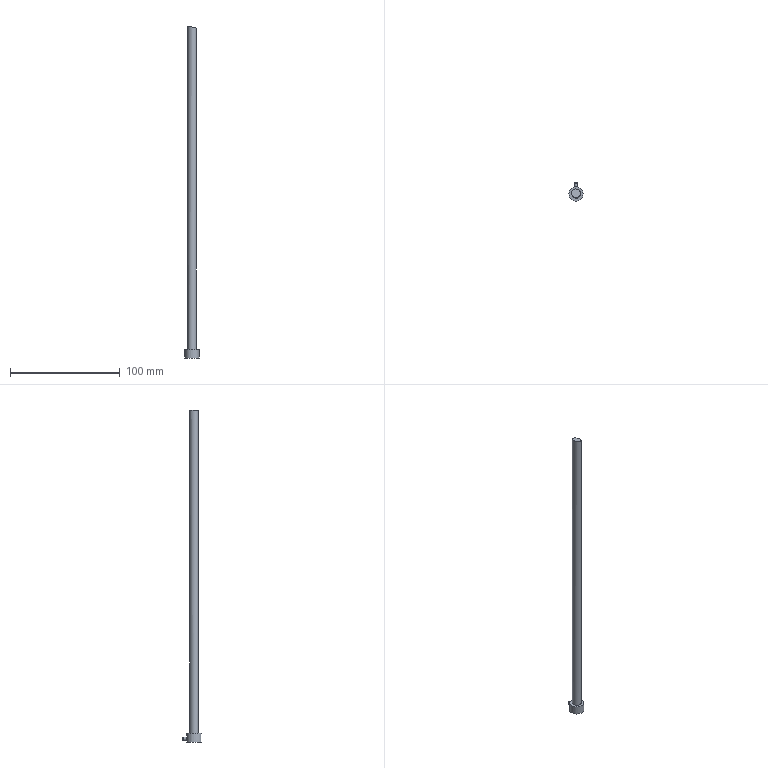Part | STEP file | E108-10-310 | 1 solid | 8 faces | box 13 x 16.5 x 302.023 mm | volume 15811 mm3 | cylinder 3 | plane 3 | spline 1 | cone 1 | commonest cylinder face diameters 3 x1 8 x1 13 x1
STEP:
#1=CARTESIAN_POINT('',(0.,0.,0.));
#2=DIRECTION('',(0.,0.,1.));
#3=DIRECTION('',(1.,0.,0.));
#4=AXIS2_PLACEMENT_3D('',#1,#2,#3);
#5=CARTESIAN_POINT('',(3.959,0.5704,299.842));
#6=VERTEX_POINT('',#5);
#7=CARTESIAN_POINT('',(3.959,0.5704,299.842));
#8=CARTESIAN_POINT('',(3.897,1.002,299.843));
#9=CARTESIAN_POINT('',(3.761,1.428,299.865));
#10=CARTESIAN_POINT('',(3.565,1.815,299.906));
#11=CARTESIAN_POINT('',(3.368,2.201,299.946));
#12=CARTESIAN_POINT('',(3.105,2.558,300.006));
#13=CARTESIAN_POINT('',(2.799,2.858,300.08));
#14=CARTESIAN_POINT('',(2.487,3.163,300.155));
#15=CARTESIAN_POINT('',(2.122,3.418,300.247));
#16=CARTESIAN_POINT('',(1.733,3.605,300.347));
#17=CARTESIAN_POINT('',(1.33,3.799,300.45));
#18=CARTESIAN_POINT('',(0.8911,3.925,300.566));
#19=CARTESIAN_POINT('',(0.4506,3.975,300.683));
#20=CARTESIAN_POINT('',(-0.003906,4.026,300.805));
#21=CARTESIAN_POINT('',(-0.4724,3.998,300.932));
#22=CARTESIAN_POINT('',(-0.9173,3.893,301.055));
#23=CARTESIAN_POINT('',(-1.369,3.787,301.18));
#24=CARTESIAN_POINT('',(-1.808,3.598,301.304));
#25=CARTESIAN_POINT('',(-2.198,3.342,301.416));
#26=CARTESIAN_POINT('',(-2.585,3.087,301.528));
#27=CARTESIAN_POINT('',(-2.934,2.759,301.632));
#28=CARTESIAN_POINT('',(-3.213,2.383,301.719));
#29=CARTESIAN_POINT('',(-3.484,2.017,301.803));
#30=CARTESIAN_POINT('',(-3.697,1.595,301.874));
#31=CARTESIAN_POINT('',(-3.83,1.154,301.925));
#32=CARTESIAN_POINT('',(-3.958,0.7275,301.974));
#33=CARTESIAN_POINT('',(-4.016,0.2708,302.006));
#34=CARTESIAN_POINT('',(-3.996,-0.1767,302.018));
#35=CARTESIAN_POINT('',(-3.977,-0.6128,302.029));
#36=CARTESIAN_POINT('',(-3.884,-1.052,302.021));
#37=CARTESIAN_POINT('',(-3.725,-1.458,301.995));
#38=CARTESIAN_POINT('',(-3.567,-1.861,301.969));
#39=CARTESIAN_POINT('',(-3.34,-2.242,301.924));
#40=CARTESIAN_POINT('',(-3.064,-2.571,301.865));
#41=CARTESIAN_POINT('',(-2.785,-2.904,301.804));
#42=CARTESIAN_POINT('',(-2.447,-3.193,301.726));
#43=CARTESIAN_POINT('',(-2.08,-3.417,301.637));
#44=CARTESIAN_POINT('',(-1.702,-3.647,301.546));
#45=CARTESIAN_POINT('',(-1.282,-3.814,301.441));
#46=CARTESIAN_POINT('',(-0.8545,-3.908,301.33));
#47=CARTESIAN_POINT('',(-0.4124,-4.004,301.215));
#48=CARTESIAN_POINT('',(0.05038,-4.025,301.091));
#49=CARTESIAN_POINT('',(0.4972,-3.969,300.968));
#50=CARTESIAN_POINT('',(0.955,-3.912,300.841));
#51=CARTESIAN_POINT('',(1.409,-3.772,300.712));
#52=CARTESIAN_POINT('',(1.821,-3.562,300.591));
#53=CARTESIAN_POINT('',(2.234,-3.35,300.469));
#54=CARTESIAN_POINT('',(2.618,-3.061,300.352));
#55=CARTESIAN_POINT('',(2.937,-2.716,300.251));
#56=CARTESIAN_POINT('',(3.249,-2.378,300.151));
#57=CARTESIAN_POINT('',(3.508,-1.978,300.064));
#58=CARTESIAN_POINT('',(3.688,-1.548,299.997));
#59=CARTESIAN_POINT('',(3.862,-1.134,299.933));
#60=CARTESIAN_POINT('',(3.967,-0.6812,299.886));
#61=CARTESIAN_POINT('',(3.993,-0.2291,299.862));
#62=CARTESIAN_POINT('',(4.009,0.03691,299.848));
#63=CARTESIAN_POINT('',(3.997,0.3063,299.841));
#64=CARTESIAN_POINT('',(3.959,0.5704,299.842));
#65=B_SPLINE_CURVE_WITH_KNOTS('',3,(#7,#8,#9,#10,#11,#12,#13,#14,#15,#16,#17,#18,#19,#20,#21,#22,#23,#24,#25,#26,#27,#28,#29,#30,#31,#32,#33,#34,#35,#36,#37,#38,#39,#40,#41,#42,#43,#44,#45,#46,#47,#48,#49,#50,#51,#52,#53,#54,#55,#56,#57,#58,#59,#60,#61,#62,#63,#64),.UNSPECIFIED.,.T.,.F.,(1,3,3,3,3,3,3,3,3,3,3,3,3,3,3,3,3,3,3,3,3,1),(-0.03113,0.,0.0513,0.1025,0.1547,0.2087,0.2644,0.321,0.3772,0.4318,0.4846,0.5361,0.5871,0.6388,0.692,0.7469,0.8033,0.8599,0.9154,0.9689,1.,1.051),.UNSPECIFIED.);
#66=CARTESIAN_POINT('',(0.,0.,108.));
#67=DIRECTION('',(0.,0.,-1.));
#68=DIRECTION('',(-1.,0.,0.));
#69=AXIS2_PLACEMENT_3D('',#66,#67,#68);
#70=CYLINDRICAL_SURFACE('',#69,4.);
#71=CARTESIAN_POINT('',(9.282,-191.842));
#72=CARTESIAN_POINT('',(9.258,-191.842));
#73=CARTESIAN_POINT('',(9.209,-191.845));
#74=CARTESIAN_POINT('',(9.136,-191.854));
#75=CARTESIAN_POINT('',(9.064,-191.87));
#76=CARTESIAN_POINT('',(8.991,-191.892));
#77=CARTESIAN_POINT('',(8.919,-191.919));
#78=CARTESIAN_POINT('',(8.847,-191.951));
#79=CARTESIAN_POINT('',(8.774,-191.989));
#80=CARTESIAN_POINT('',(8.702,-192.031));
#81=CARTESIAN_POINT('',(8.631,-192.078));
#82=CARTESIAN_POINT('',(8.559,-192.13));
#83=CARTESIAN_POINT('',(8.488,-192.185));
#84=CARTESIAN_POINT('',(8.416,-192.245));
#85=CARTESIAN_POINT('',(8.345,-192.307));
#86=CARTESIAN_POINT('',(8.275,-192.372));
#87=CARTESIAN_POINT('',(8.204,-192.44));
#88=CARTESIAN_POINT('',(8.133,-192.51));
#89=CARTESIAN_POINT('',(8.063,-192.583));
#90=CARTESIAN_POINT('',(7.992,-192.656));
#91=CARTESIAN_POINT('',(7.922,-192.731));
#92=CARTESIAN_POINT('',(7.852,-192.806));
#93=CARTESIAN_POINT('',(7.782,-192.883));
#94=CARTESIAN_POINT('',(7.712,-192.959));
#95=CARTESIAN_POINT('',(7.641,-193.035));
#96=CARTESIAN_POINT('',(7.572,-193.11));
#97=CARTESIAN_POINT('',(7.501,-193.185));
#98=CARTESIAN_POINT('',(7.431,-193.258));
#99=CARTESIAN_POINT('',(7.36,-193.33));
#100=CARTESIAN_POINT('',(7.29,-193.4));
#101=CARTESIAN_POINT('',(7.22,-193.467));
#102=CARTESIAN_POINT('',(7.149,-193.532));
#103=CARTESIAN_POINT('',(7.077,-193.594));
#104=CARTESIAN_POINT('',(7.006,-193.653));
#105=CARTESIAN_POINT('',(6.935,-193.709));
#106=CARTESIAN_POINT('',(6.864,-193.761));
#107=CARTESIAN_POINT('',(6.792,-193.808));
#108=CARTESIAN_POINT('',(6.72,-193.852));
#109=CARTESIAN_POINT('',(6.648,-193.891));
#110=CARTESIAN_POINT('',(6.576,-193.926));
#111=CARTESIAN_POINT('',(6.504,-193.955));
#112=CARTESIAN_POINT('',(6.431,-193.98));
#113=CARTESIAN_POINT('',(6.359,-193.999));
#114=CARTESIAN_POINT('',(6.286,-194.013));
#115=CARTESIAN_POINT('',(6.214,-194.021));
#116=CARTESIAN_POINT('',(6.141,-194.024));
#117=CARTESIAN_POINT('',(6.068,-194.021));
#118=CARTESIAN_POINT('',(5.995,-194.013));
#119=CARTESIAN_POINT('',(5.923,-193.999));
#120=CARTESIAN_POINT('',(5.85,-193.98));
#121=CARTESIAN_POINT('',(5.778,-193.955));
#122=CARTESIAN_POINT('',(5.705,-193.926));
#123=CARTESIAN_POINT('',(5.633,-193.891));
#124=CARTESIAN_POINT('',(5.561,-193.852));
#125=CARTESIAN_POINT('',(5.489,-193.808));
#126=CARTESIAN_POINT('',(5.417,-193.759));
#127=CARTESIAN_POINT('',(5.345,-193.706));
#128=CARTESIAN_POINT('',(5.274,-193.65));
#129=CARTESIAN_POINT('',(5.203,-193.591));
#130=CARTESIAN_POINT('',(5.132,-193.528));
#131=CARTESIAN_POINT('',(5.061,-193.462));
#132=CARTESIAN_POINT('',(4.99,-193.393));
#133=CARTESIAN_POINT('',(4.92,-193.322));
#134=CARTESIAN_POINT('',(4.85,-193.25));
#135=CARTESIAN_POINT('',(4.779,-193.176));
#136=CARTESIAN_POINT('',(4.709,-193.1));
#137=CARTESIAN_POINT('',(4.639,-193.024));
#138=CARTESIAN_POINT('',(4.569,-192.947));
#139=CARTESIAN_POINT('',(4.499,-192.87));
#140=CARTESIAN_POINT('',(4.429,-192.793));
#141=CARTESIAN_POINT('',(4.358,-192.717));
#142=CARTESIAN_POINT('',(4.288,-192.642));
#143=CARTESIAN_POINT('',(4.218,-192.568));
#144=CARTESIAN_POINT('',(4.148,-192.496));
#145=CARTESIAN_POINT('',(4.077,-192.425));
#146=CARTESIAN_POINT('',(4.006,-192.357));
#147=CARTESIAN_POINT('',(3.936,-192.292));
#148=CARTESIAN_POINT('',(3.865,-192.23));
#149=CARTESIAN_POINT('',(3.794,-192.172));
#150=CARTESIAN_POINT('',(3.722,-192.117));
#151=CARTESIAN_POINT('',(3.651,-192.066));
#152=CARTESIAN_POINT('',(3.579,-192.02));
#153=CARTESIAN_POINT('',(3.507,-191.979));
#154=CARTESIAN_POINT('',(3.435,-191.942));
#155=CARTESIAN_POINT('',(3.363,-191.911));
#156=CARTESIAN_POINT('',(3.29,-191.885));
#157=CARTESIAN_POINT('',(3.218,-191.865));
#158=CARTESIAN_POINT('',(3.145,-191.851));
#159=CARTESIAN_POINT('',(3.072,-191.843));
#160=CARTESIAN_POINT('',(3.023,-191.841));
#161=CARTESIAN_POINT('',(2.999,-191.842));
#162=B_SPLINE_CURVE_WITH_KNOTS('',3,(#71,#72,#73,#74,#75,#76,#77,#78,#79,#80,#81,#82,#83,#84,#85,#86,#87,#88,#89,#90,#91,#92,#93,#94,#95,#96,#97,#98,#99,#100,#101,#102,#103,#104,#105,#106,#107,#108,#109,#110,#111,#112,#113,#114,#115,#116,#117,#118,#119,#120,#121,#122,#123,#124,#125,#126,#127,#128,#129,#130,#131,#132,#133,#134,#135,#136,#137,#138,#139,#140,#141,#142,#143,#144,#145,#146,#147,#148,#149,#150,#151,#152,#153,#154,#155,#156,#157,#158,#159,#160,#161),.UNSPECIFIED.,.F.,.F.,(4,1,1,1,1,1,1,1,1,1,1,1,1,1,1,1,1,1,1,1,1,1,1,1,1,1,1,1,1,1,1,1,1,1,1,1,1,1,1,1,1,1,1,1,1,1,1,1,1,1,1,1,1,1,1,1,1,1,1,1,1,1,1,1,1,1,1,1,1,1,1,1,1,1,1,1,1,1,1,1,1,1,1,1,1,1,1,1,4),(0.,0.01136,0.02273,0.03409,0.04545,0.05682,0.06818,0.07955,0.09091,0.1023,0.1136,0.125,0.1364,0.1477,0.1591,0.1705,0.1818,0.1932,0.2045,0.2159,0.2273,0.2386,0.25,0.2614,0.2727,0.2841,0.2955,0.3068,0.3182,0.3295,0.3409,0.3523,0.3636,0.375,0.3864,0.3977,0.4091,0.4205,0.4318,0.4432,0.4545,0.4659,0.4773,0.4886,0.5,0.5114,0.5227,0.5341,0.5455,0.5568,0.5682,0.5795,0.5909,0.6023,0.6136,0.625,0.6364,0.6477,0.6591,0.6705,0.6818,0.6932,0.7045,0.7159,0.7273,0.7386,0.75,0.7614,0.7727,0.7841,0.7955,0.8068,0.8182,0.8295,0.8409,0.8523,0.8636,0.875,0.8864,0.8977,0.9091,0.9205,0.9318,0.9432,0.9545,0.9659,0.9773,0.9886,1.),.QUASI_UNIFORM_KNOTS.);
#163=(GEOMETRIC_REPRESENTATION_CONTEXT(2)PARAMETRIC_REPRESENTATION_CONTEXT()REPRESENTATION_CONTEXT('',''));
#164=DEFINITIONAL_REPRESENTATION('',(#162),#163);
#165=PCURVE('',#70,#164);
#166=CARTESIAN_POINT('',(-6.783,-9.336,303.066));
#167=CARTESIAN_POINT('',(-2.101,-9.334,301.894));
#168=CARTESIAN_POINT('',(2.631,-9.333,300.612));
#169=CARTESIAN_POINT('',(7.412,-9.331,299.224));
#170=CARTESIAN_POINT('',(-6.847,-4.458,302.903));
#171=CARTESIAN_POINT('',(-2.168,-4.457,301.732));
#172=CARTESIAN_POINT('',(2.56,-4.456,300.452));
#173=CARTESIAN_POINT('',(7.338,-4.454,299.065));
#174=CARTESIAN_POINT('',(-6.914,0.4188,302.739));
#175=CARTESIAN_POINT('',(-2.239,0.4202,301.569));
#176=CARTESIAN_POINT('',(2.486,0.4215,300.29));
#177=CARTESIAN_POINT('',(7.261,0.4227,298.904));
#178=CARTESIAN_POINT('',(-6.985,5.296,302.573));
#179=CARTESIAN_POINT('',(-2.312,5.297,301.405));
#180=CARTESIAN_POINT('',(2.41,5.298,300.127));
#181=CARTESIAN_POINT('',(7.182,5.3,298.743));
#182=B_SPLINE_SURFACE_WITH_KNOTS('',3,3,((#166,#167,#168,#169),(#170,#171,#172,#173),(#174,#175,#176,#177),(#178,#179,#180,#181)),.UNSPECIFIED.,.F.,.F.,.F.,(4,4),(4,4),(0.,1.),(0.,1.),.PIECEWISE_BEZIER_KNOTS.);
#183=CARTESIAN_POINT('',(0.6768,0.7691));
#184=CARTESIAN_POINT('',(0.6833,0.7683));
#185=CARTESIAN_POINT('',(0.6964,0.7661));
#186=CARTESIAN_POINT('',(0.7157,0.7612));
#187=CARTESIAN_POINT('',(0.7345,0.755));
#188=CARTESIAN_POINT('',(0.7529,0.7475));
#189=CARTESIAN_POINT('',(0.7704,0.7386));
#190=CARTESIAN_POINT('',(0.7874,0.7283));
#191=CARTESIAN_POINT('',(0.8035,0.7169));
#192=CARTESIAN_POINT('',(0.8188,0.7043));
#193=CARTESIAN_POINT('',(0.833,0.6907));
#194=CARTESIAN_POINT('',(0.8462,0.676));
#195=CARTESIAN_POINT('',(0.8583,0.6604));
#196=CARTESIAN_POINT('',(0.8693,0.644));
#197=CARTESIAN_POINT('',(0.8791,0.6269));
#198=CARTESIAN_POINT('',(0.8876,0.6091));
#199=CARTESIAN_POINT('',(0.8949,0.5908));
#200=CARTESIAN_POINT('',(0.9009,0.5719));
#201=CARTESIAN_POINT('',(0.9056,0.5527));
#202=CARTESIAN_POINT('',(0.9089,0.5332));
#203=CARTESIAN_POINT('',(0.9109,0.5136));
#204=CARTESIAN_POINT('',(0.9115,0.4938));
#205=CARTESIAN_POINT('',(0.9108,0.4739));
#206=CARTESIAN_POINT('',(0.9087,0.4541));
#207=CARTESIAN_POINT('',(0.9054,0.4345));
#208=CARTESIAN_POINT('',(0.9007,0.4153));
#209=CARTESIAN_POINT('',(0.8947,0.3963));
#210=CARTESIAN_POINT('',(0.8874,0.3777));
#211=CARTESIAN_POINT('',(0.8789,0.3597));
#212=CARTESIAN_POINT('',(0.8692,0.3423));
#213=CARTESIAN_POINT('',(0.8583,0.3257));
#214=CARTESIAN_POINT('',(0.8463,0.3097));
#215=CARTESIAN_POINT('',(0.8331,0.2946));
#216=CARTESIAN_POINT('',(0.819,0.2805));
#217=CARTESIAN_POINT('',(0.804,0.2674));
#218=CARTESIAN_POINT('',(0.7881,0.2555));
#219=CARTESIAN_POINT('',(0.7713,0.2447));
#220=CARTESIAN_POINT('',(0.7537,0.2352));
#221=CARTESIAN_POINT('',(0.7356,0.2269));
#222=CARTESIAN_POINT('',(0.717,0.22));
#223=CARTESIAN_POINT('',(0.6979,0.2145));
#224=CARTESIAN_POINT('',(0.6783,0.2105));
#225=CARTESIAN_POINT('',(0.6586,0.2078));
#226=CARTESIAN_POINT('',(0.6387,0.2067));
#227=CARTESIAN_POINT('',(0.6189,0.2071));
#228=CARTESIAN_POINT('',(0.5992,0.209));
#229=CARTESIAN_POINT('',(0.5795,0.2124));
#230=CARTESIAN_POINT('',(0.5602,0.2173));
#231=CARTESIAN_POINT('',(0.5414,0.2235));
#232=CARTESIAN_POINT('',(0.5232,0.2312));
#233=CARTESIAN_POINT('',(0.5055,0.2403));
#234=CARTESIAN_POINT('',(0.4885,0.2507));
#235=CARTESIAN_POINT('',(0.4723,0.2622));
#236=CARTESIAN_POINT('',(0.4571,0.2749));
#237=CARTESIAN_POINT('',(0.4428,0.2887));
#238=CARTESIAN_POINT('',(0.4296,0.3036));
#239=CARTESIAN_POINT('',(0.4174,0.3193));
#240=CARTESIAN_POINT('',(0.4064,0.3358));
#241=CARTESIAN_POINT('',(0.3967,0.353));
#242=CARTESIAN_POINT('',(0.3881,0.371));
#243=CARTESIAN_POINT('',(0.3808,0.3895));
#244=CARTESIAN_POINT('',(0.3748,0.4085));
#245=CARTESIAN_POINT('',(0.3702,0.4277));
#246=CARTESIAN_POINT('',(0.3669,0.4472));
#247=CARTESIAN_POINT('',(0.3649,0.467));
#248=CARTESIAN_POINT('',(0.3643,0.4868));
#249=CARTESIAN_POINT('',(0.365,0.5066));
#250=CARTESIAN_POINT('',(0.3671,0.5262));
#251=CARTESIAN_POINT('',(0.3705,0.5457));
#252=CARTESIAN_POINT('',(0.3752,0.565));
#253=CARTESIAN_POINT('',(0.3813,0.5839));
#254=CARTESIAN_POINT('',(0.3885,0.6023));
#255=CARTESIAN_POINT('',(0.397,0.6201));
#256=CARTESIAN_POINT('',(0.4067,0.6373));
#257=CARTESIAN_POINT('',(0.4176,0.6539));
#258=CARTESIAN_POINT('',(0.4297,0.6696));
#259=CARTESIAN_POINT('',(0.4427,0.6846));
#260=CARTESIAN_POINT('',(0.4567,0.6984));
#261=CARTESIAN_POINT('',(0.4718,0.7113));
#262=CARTESIAN_POINT('',(0.4878,0.7232));
#263=CARTESIAN_POINT('',(0.5045,0.7339));
#264=CARTESIAN_POINT('',(0.522,0.7434));
#265=CARTESIAN_POINT('',(0.54,0.7515));
#266=CARTESIAN_POINT('',(0.5587,0.7583));
#267=CARTESIAN_POINT('',(0.5778,0.7638));
#268=CARTESIAN_POINT('',(0.5974,0.7679));
#269=CARTESIAN_POINT('',(0.617,0.7705));
#270=CARTESIAN_POINT('',(0.6369,0.7716));
#271=CARTESIAN_POINT('',(0.657,0.7713));
#272=CARTESIAN_POINT('',(0.6702,0.77));
#273=CARTESIAN_POINT('',(0.6768,0.7691));
#274=B_SPLINE_CURVE_WITH_KNOTS('',3,(#183,#184,#185,#186,#187,#188,#189,#190,#191,#192,#193,#194,#195,#196,#197,#198,#199,#200,#201,#202,#203,#204,#205,#206,#207,#208,#209,#210,#211,#212,#213,#214,#215,#216,#217,#218,#219,#220,#221,#222,#223,#224,#225,#226,#227,#228,#229,#230,#231,#232,#233,#234,#235,#236,#237,#238,#239,#240,#241,#242,#243,#244,#245,#246,#247,#248,#249,#250,#251,#252,#253,#254,#255,#256,#257,#258,#259,#260,#261,#262,#263,#264,#265,#266,#267,#268,#269,#270,#271,#272,#273),.UNSPECIFIED.,.T.,.F.,(4,1,1,1,1,1,1,1,1,1,1,1,1,1,1,1,1,1,1,1,1,1,1,1,1,1,1,1,1,1,1,1,1,1,1,1,1,1,1,1,1,1,1,1,1,1,1,1,1,1,1,1,1,1,1,1,1,1,1,1,1,1,1,1,1,1,1,1,1,1,1,1,1,1,1,1,1,1,1,1,1,1,1,1,1,1,1,1,4),(0.,0.01136,0.02273,0.03409,0.04545,0.05682,0.06818,0.07955,0.09091,0.1023,0.1136,0.125,0.1364,0.1477,0.1591,0.1705,0.1818,0.1932,0.2045,0.2159,0.2273,0.2386,0.25,0.2614,0.2727,0.2841,0.2955,0.3068,0.3182,0.3295,0.3409,0.3523,0.3636,0.375,0.3864,0.3977,0.4091,0.4205,0.4318,0.4432,0.4545,0.4659,0.4773,0.4886,0.5,0.5114,0.5227,0.5341,0.5455,0.5568,0.5682,0.5795,0.5909,0.6023,0.6136,0.625,0.6364,0.6477,0.6591,0.6705,0.6818,0.6932,0.7045,0.7159,0.7273,0.7386,0.75,0.7614,0.7727,0.7841,0.7955,0.8068,0.8182,0.8295,0.8409,0.8523,0.8636,0.875,0.8864,0.8977,0.9091,0.9205,0.9318,0.9432,0.9545,0.9659,0.9773,0.9886,1.),.QUASI_UNIFORM_KNOTS.);
#275=(GEOMETRIC_REPRESENTATION_CONTEXT(2)PARAMETRIC_REPRESENTATION_CONTEXT()REPRESENTATION_CONTEXT('',''));
#276=DEFINITIONAL_REPRESENTATION('',(#274),#275);
#277=PCURVE('',#182,#276);
#278=SURFACE_CURVE('',#65,(#165,#277),.PCURVE_S1.);
#279=EDGE_CURVE('',#6,#6,#278,.T.);
#280=ORIENTED_EDGE('',*,*,#279,.F.);
#281=CARTESIAN_POINT('',(3.959,0.5704,8.));
#282=VERTEX_POINT('',#281);
#283=CARTESIAN_POINT('',(3.959,0.5704,299.842));
#284=CARTESIAN_POINT('',(3.959,0.5704,8.));
#285=B_SPLINE_CURVE_WITH_KNOTS('',1,(#283,#284),.UNSPECIFIED.,.F.,.F.,(2,2),(-191.842,100.),.PIECEWISE_BEZIER_KNOTS.);
#286=CARTESIAN_POINT('',(9.282,0.));
#287=DIRECTION('',(0.,1.));
#288=VECTOR('',#287,1.);
#289=LINE('',#286,#288);
#290=(GEOMETRIC_REPRESENTATION_CONTEXT(2)PARAMETRIC_REPRESENTATION_CONTEXT()REPRESENTATION_CONTEXT('',''));
#291=DEFINITIONAL_REPRESENTATION('',(#289),#290);
#292=PCURVE('',#70,#291);
#293=CARTESIAN_POINT('',(2.999,0.));
#294=DIRECTION('',(0.,1.));
#295=VECTOR('',#294,1.);
#296=LINE('',#293,#295);
#297=(GEOMETRIC_REPRESENTATION_CONTEXT(2)PARAMETRIC_REPRESENTATION_CONTEXT()REPRESENTATION_CONTEXT('',''));
#298=DEFINITIONAL_REPRESENTATION('',(#296),#297);
#299=PCURVE('',#70,#298);
#300=SEAM_CURVE('',#285,(#292,#299),.PCURVE_S1.);
#301=EDGE_CURVE('',#6,#282,#300,.T.);
#302=ORIENTED_EDGE('',*,*,#301,.T.);
#303=CARTESIAN_POINT('',(4.,0.,8.));
#304=VERTEX_POINT('',#303);
#305=CARTESIAN_POINT('',(0.,0.,8.));
#306=DIRECTION('',(0.,0.,1.));
#307=DIRECTION('',(1.,0.,0.));
#308=AXIS2_PLACEMENT_3D('',#305,#306,#307);
#309=CIRCLE('',#308,4.);
#310=CARTESIAN_POINT('',(9.425,100.));
#311=DIRECTION('',(-1.,0.));
#312=VECTOR('',#311,1.);
#313=LINE('',#310,#312);
#314=(GEOMETRIC_REPRESENTATION_CONTEXT(2)PARAMETRIC_REPRESENTATION_CONTEXT()REPRESENTATION_CONTEXT('',''));
#315=DEFINITIONAL_REPRESENTATION('',(#313),#314);
#316=PCURVE('',#70,#315);
#317=CARTESIAN_POINT('',(0.,0.,8.));
#318=DIRECTION('',(0.,0.,-1.));
#319=DIRECTION('',(1.,0.,0.));
#320=AXIS2_PLACEMENT_3D('',#317,#318,#319);
#321=PLANE('',#320);
#322=CARTESIAN_POINT('',(4.,0.));
#323=CARTESIAN_POINT('',(4.,-6.928));
#324=CARTESIAN_POINT('',(-2.,-3.464));
#325=CARTESIAN_POINT('',(-8.,0.));
#326=CARTESIAN_POINT('',(-2.,3.464));
#327=CARTESIAN_POINT('',(4.,6.928));
#328=CARTESIAN_POINT('',(4.,0.));
#329=(BOUNDED_CURVE()B_SPLINE_CURVE(2,(#322,#323,#324,#325,#326,#327,#328),.UNSPECIFIED.,.T.,.F.)B_SPLINE_CURVE_WITH_KNOTS((1,2,2,2,2,1),(-2.094,0.,2.094,4.189,6.283,8.378),.UNSPECIFIED.)CURVE()GEOMETRIC_REPRESENTATION_ITEM()RATIONAL_B_SPLINE_CURVE((1.,0.5,1.,0.5,1.,0.5,1.))REPRESENTATION_ITEM(''));
#330=(GEOMETRIC_REPRESENTATION_CONTEXT(2)PARAMETRIC_REPRESENTATION_CONTEXT()REPRESENTATION_CONTEXT('',''));
#331=DEFINITIONAL_REPRESENTATION('',(#329),#330);
#332=PCURVE('',#321,#331);
#333=SURFACE_CURVE('',#309,(#316,#332),.PCURVE_S1.);
#334=EDGE_CURVE('',#282,#304,#333,.T.);
#335=ORIENTED_EDGE('',*,*,#334,.T.);
#336=CARTESIAN_POINT('',(0.,0.,8.));
#337=DIRECTION('',(0.,0.,1.));
#338=DIRECTION('',(1.,0.,0.));
#339=AXIS2_PLACEMENT_3D('',#336,#337,#338);
#340=CIRCLE('',#339,4.);
#341=CARTESIAN_POINT('',(3.142,100.));
#342=DIRECTION('',(-1.,0.));
#343=VECTOR('',#342,1.);
#344=LINE('',#341,#343);
#345=(GEOMETRIC_REPRESENTATION_CONTEXT(2)PARAMETRIC_REPRESENTATION_CONTEXT()REPRESENTATION_CONTEXT('',''));
#346=DEFINITIONAL_REPRESENTATION('',(#344),#345);
#347=PCURVE('',#70,#346);
#348=CARTESIAN_POINT('',(4.,0.));
#349=CARTESIAN_POINT('',(4.,-6.928));
#350=CARTESIAN_POINT('',(-2.,-3.464));
#351=CARTESIAN_POINT('',(-8.,0.));
#352=CARTESIAN_POINT('',(-2.,3.464));
#353=CARTESIAN_POINT('',(4.,6.928));
#354=CARTESIAN_POINT('',(4.,0.));
#355=(BOUNDED_CURVE()B_SPLINE_CURVE(2,(#348,#349,#350,#351,#352,#353,#354),.UNSPECIFIED.,.T.,.F.)B_SPLINE_CURVE_WITH_KNOTS((1,2,2,2,2,1),(-2.094,0.,2.094,4.189,6.283,8.378),.UNSPECIFIED.)CURVE()GEOMETRIC_REPRESENTATION_ITEM()RATIONAL_B_SPLINE_CURVE((1.,0.5,1.,0.5,1.,0.5,1.))REPRESENTATION_ITEM(''));
#356=(GEOMETRIC_REPRESENTATION_CONTEXT(2)PARAMETRIC_REPRESENTATION_CONTEXT()REPRESENTATION_CONTEXT('',''));
#357=DEFINITIONAL_REPRESENTATION('',(#355),#356);
#358=PCURVE('',#321,#357);
#359=SURFACE_CURVE('',#340,(#347,#358),.PCURVE_S1.);
#360=EDGE_CURVE('',#304,#282,#359,.T.);
#361=ORIENTED_EDGE('',*,*,#360,.T.);
#362=ORIENTED_EDGE('',*,*,#301,.F.);
#363=EDGE_LOOP('',(#280,#302,#335,#361,#362));
#364=FACE_BOUND('',#363,.T.);
#365=ADVANCED_FACE('',(#364),#70,.T.);
#366=ORIENTED_EDGE('',*,*,#279,.F.);
#367=EDGE_LOOP('',(#366));
#368=FACE_BOUND('',#367,.F.);
#369=ADVANCED_FACE('',(#368),#182,.F.);
#370=CARTESIAN_POINT('',(6.5,0.,0.));
#371=VERTEX_POINT('',#370);
#372=CARTESIAN_POINT('',(-6.5,0.,0.));
#373=VERTEX_POINT('',#372);
#374=CARTESIAN_POINT('',(0.,0.,0.));
#375=DIRECTION('',(0.,0.,-1.));
#376=DIRECTION('',(-1.,0.,0.));
#377=AXIS2_PLACEMENT_3D('',#374,#375,#376);
#378=CIRCLE('',#377,6.5);
#379=CARTESIAN_POINT('',(0.,0.,8.));
#380=DIRECTION('',(0.,0.,-1.));
#381=DIRECTION('',(1.,0.,0.));
#382=AXIS2_PLACEMENT_3D('',#379,#380,#381);
#383=CYLINDRICAL_SURFACE('',#382,6.5);
#384=CARTESIAN_POINT('',(-3.142,8.));
#385=DIRECTION('',(1.,0.));
#386=VECTOR('',#385,1.);
#387=LINE('',#384,#386);
#388=(GEOMETRIC_REPRESENTATION_CONTEXT(2)PARAMETRIC_REPRESENTATION_CONTEXT()REPRESENTATION_CONTEXT('',''));
#389=DEFINITIONAL_REPRESENTATION('',(#387),#388);
#390=PCURVE('',#383,#389);
#391=CARTESIAN_POINT('',(240.,-1000.,0.));
#392=DIRECTION('',(0.,0.,1.));
#393=DIRECTION('',(-1.,0.,0.));
#394=AXIS2_PLACEMENT_3D('',#391,#392,#393);
#395=PLANE('',#394);
#396=CARTESIAN_POINT('',(246.5,-1000.));
#397=CARTESIAN_POINT('',(246.5,-1011.258));
#398=CARTESIAN_POINT('',(236.75,-1005.629));
#399=CARTESIAN_POINT('',(227.,-1000.));
#400=CARTESIAN_POINT('',(236.75,-994.371));
#401=CARTESIAN_POINT('',(246.5,-988.742));
#402=CARTESIAN_POINT('',(246.5,-1000.));
#403=(BOUNDED_CURVE()B_SPLINE_CURVE(2,(#396,#397,#398,#399,#400,#401,#402),.UNSPECIFIED.,.T.,.F.)B_SPLINE_CURVE_WITH_KNOTS((1,2,2,2,2,1),(-2.094,0.,2.094,4.189,6.283,8.378),.UNSPECIFIED.)CURVE()GEOMETRIC_REPRESENTATION_ITEM()RATIONAL_B_SPLINE_CURVE((1.,0.5,1.,0.5,1.,0.5,1.))REPRESENTATION_ITEM(''));
#404=(GEOMETRIC_REPRESENTATION_CONTEXT(2)PARAMETRIC_REPRESENTATION_CONTEXT()REPRESENTATION_CONTEXT('',''));
#405=DEFINITIONAL_REPRESENTATION('',(#403),#404);
#406=PCURVE('',#395,#405);
#407=SURFACE_CURVE('',#378,(#390,#406),.PCURVE_S1.);
#408=EDGE_CURVE('',#371,#373,#407,.T.);
#409=ORIENTED_EDGE('',*,*,#408,.F.);
#410=CARTESIAN_POINT('',(6.5,0.,8.));
#411=VERTEX_POINT('',#410);
#412=CARTESIAN_POINT('',(6.5,0.,8.));
#413=CARTESIAN_POINT('',(6.5,0.,0.));
#414=B_SPLINE_CURVE_WITH_KNOTS('',1,(#412,#413),.UNSPECIFIED.,.F.,.F.,(2,2),(0.,8.),.PIECEWISE_BEZIER_KNOTS.);
#415=CARTESIAN_POINT('',(0.,0.));
#416=DIRECTION('',(0.,1.));
#417=VECTOR('',#416,1.);
#418=LINE('',#415,#417);
#419=(GEOMETRIC_REPRESENTATION_CONTEXT(2)PARAMETRIC_REPRESENTATION_CONTEXT()REPRESENTATION_CONTEXT('',''));
#420=DEFINITIONAL_REPRESENTATION('',(#418),#419);
#421=PCURVE('',#383,#420);
#422=CARTESIAN_POINT('',(6.283,0.));
#423=DIRECTION('',(0.,1.));
#424=VECTOR('',#423,1.);
#425=LINE('',#422,#424);
#426=(GEOMETRIC_REPRESENTATION_CONTEXT(2)PARAMETRIC_REPRESENTATION_CONTEXT()REPRESENTATION_CONTEXT('',''));
#427=DEFINITIONAL_REPRESENTATION('',(#425),#426);
#428=PCURVE('',#383,#427);
#429=SEAM_CURVE('',#414,(#421,#428),.PCURVE_S1.);
#430=EDGE_CURVE('',#411,#371,#429,.T.);
#431=ORIENTED_EDGE('',*,*,#430,.F.);
#432=CARTESIAN_POINT('',(0.,0.,8.));
#433=DIRECTION('',(0.,0.,-1.));
#434=DIRECTION('',(1.,0.,0.));
#435=AXIS2_PLACEMENT_3D('',#432,#433,#434);
#436=CIRCLE('',#435,6.5);
#437=CARTESIAN_POINT('',(0.,0.));
#438=DIRECTION('',(1.,0.));
#439=VECTOR('',#438,1.);
#440=LINE('',#437,#439);
#441=(GEOMETRIC_REPRESENTATION_CONTEXT(2)PARAMETRIC_REPRESENTATION_CONTEXT()REPRESENTATION_CONTEXT('',''));
#442=DEFINITIONAL_REPRESENTATION('',(#440),#441);
#443=PCURVE('',#383,#442);
#444=CARTESIAN_POINT('',(0.,0.));
#445=DIRECTION('',(1.,0.));
#446=AXIS2_PLACEMENT_2D('',#444,#445);
#447=CIRCLE('',#446,6.5);
#448=(GEOMETRIC_REPRESENTATION_CONTEXT(2)PARAMETRIC_REPRESENTATION_CONTEXT()REPRESENTATION_CONTEXT('',''));
#449=DEFINITIONAL_REPRESENTATION('',(#447),#448);
#450=PCURVE('',#321,#449);
#451=SURFACE_CURVE('',#436,(#443,#450),.PCURVE_S1.);
#452=EDGE_CURVE('',#411,#411,#451,.T.);
#453=ORIENTED_EDGE('',*,*,#452,.T.);
#454=ORIENTED_EDGE('',*,*,#430,.T.);
#455=CARTESIAN_POINT('',(0.,0.,0.));
#456=DIRECTION('',(0.,0.,-1.));
#457=DIRECTION('',(-1.,0.,0.));
#458=AXIS2_PLACEMENT_3D('',#455,#456,#457);
#459=CIRCLE('',#458,6.5);
#460=CARTESIAN_POINT('',(3.142,8.));
#461=DIRECTION('',(1.,0.));
#462=VECTOR('',#461,1.);
#463=LINE('',#460,#462);
#464=(GEOMETRIC_REPRESENTATION_CONTEXT(2)PARAMETRIC_REPRESENTATION_CONTEXT()REPRESENTATION_CONTEXT('',''));
#465=DEFINITIONAL_REPRESENTATION('',(#463),#464);
#466=PCURVE('',#383,#465);
#467=CARTESIAN_POINT('',(246.5,-1000.));
#468=CARTESIAN_POINT('',(246.5,-1011.258));
#469=CARTESIAN_POINT('',(236.75,-1005.629));
#470=CARTESIAN_POINT('',(227.,-1000.));
#471=CARTESIAN_POINT('',(236.75,-994.371));
#472=CARTESIAN_POINT('',(246.5,-988.742));
#473=CARTESIAN_POINT('',(246.5,-1000.));
#474=(BOUNDED_CURVE()B_SPLINE_CURVE(2,(#467,#468,#469,#470,#471,#472,#473),.UNSPECIFIED.,.T.,.F.)B_SPLINE_CURVE_WITH_KNOTS((1,2,2,2,2,1),(-2.094,0.,2.094,4.189,6.283,8.378),.UNSPECIFIED.)CURVE()GEOMETRIC_REPRESENTATION_ITEM()RATIONAL_B_SPLINE_CURVE((1.,0.5,1.,0.5,1.,0.5,1.))REPRESENTATION_ITEM(''));
#475=(GEOMETRIC_REPRESENTATION_CONTEXT(2)PARAMETRIC_REPRESENTATION_CONTEXT()REPRESENTATION_CONTEXT('',''));
#476=DEFINITIONAL_REPRESENTATION('',(#474),#475);
#477=PCURVE('',#395,#476);
#478=SURFACE_CURVE('',#459,(#466,#477),.PCURVE_S1.);
#479=EDGE_CURVE('',#373,#371,#478,.T.);
#480=ORIENTED_EDGE('',*,*,#479,.F.);
#481=EDGE_LOOP('',(#409,#431,#453,#454,#480));
#482=FACE_BOUND('',#481,.T.);
#483=CARTESIAN_POINT('',(0.,6.5,1.5));
#484=VERTEX_POINT('',#483);
#485=CARTESIAN_POINT('',(0.,6.5,1.5));
#486=CARTESIAN_POINT('',(0.1654,6.5,1.5));
#487=CARTESIAN_POINT('',(0.3332,6.493,1.528));
#488=CARTESIAN_POINT('',(0.4892,6.482,1.582));
#489=CARTESIAN_POINT('',(0.6451,6.47,1.636));
#490=CARTESIAN_POINT('',(0.7936,6.453,1.717));
#491=CARTESIAN_POINT('',(0.9231,6.434,1.818));
#492=CARTESIAN_POINT('',(1.055,6.415,1.92));
#493=CARTESIAN_POINT('',(1.17,6.394,2.047));
#494=CARTESIAN_POINT('',(1.261,6.377,2.187));
#495=CARTESIAN_POINT('',(1.352,6.358,2.329));
#496=CARTESIAN_POINT('',(1.421,6.343,2.49));
#497=CARTESIAN_POINT('',(1.46,6.334,2.655));
#498=CARTESIAN_POINT('',(1.498,6.325,2.817));
#499=CARTESIAN_POINT('',(1.509,6.322,2.989));
#500=CARTESIAN_POINT('',(1.492,6.326,3.155));
#501=CARTESIAN_POINT('',(1.475,6.33,3.318));
#502=CARTESIAN_POINT('',(1.431,6.341,3.48));
#503=CARTESIAN_POINT('',(1.362,6.356,3.628));
#504=CARTESIAN_POINT('',(1.293,6.37,3.777));
#505=CARTESIAN_POINT('',(1.199,6.39,3.917));
#506=CARTESIAN_POINT('',(1.085,6.409,4.035));
#507=CARTESIAN_POINT('',(0.9695,6.428,4.157));
#508=CARTESIAN_POINT('',(0.8309,6.448,4.26));
#509=CARTESIAN_POINT('',(0.6809,6.464,4.337));
#510=CARTESIAN_POINT('',(0.5305,6.48,4.413));
#511=CARTESIAN_POINT('',(0.3642,6.492,4.465));
#512=CARTESIAN_POINT('',(0.1962,6.497,4.487));
#513=CARTESIAN_POINT('',(0.03191,6.502,4.509));
#514=CARTESIAN_POINT('',(-0.1386,6.501,4.503));
#515=CARTESIAN_POINT('',(-0.3008,6.493,4.47));
#516=CARTESIAN_POINT('',(-0.4611,6.486,4.437));
#517=CARTESIAN_POINT('',(-0.6177,6.472,4.377));
#518=CARTESIAN_POINT('',(-0.7583,6.456,4.294));
#519=CARTESIAN_POINT('',(-0.9011,6.439,4.211));
#520=CARTESIAN_POINT('',(-1.031,6.419,4.102));
#521=CARTESIAN_POINT('',(-1.139,6.399,3.976));
#522=CARTESIAN_POINT('',(-1.249,6.38,3.848));
#523=CARTESIAN_POINT('',(-1.338,6.361,3.699));
#524=CARTESIAN_POINT('',(-1.399,6.348,3.541));
#525=CARTESIAN_POINT('',(-1.46,6.334,3.384));
#526=CARTESIAN_POINT('',(-1.494,6.326,3.214));
#527=CARTESIAN_POINT('',(-1.499,6.325,3.046));
#528=CARTESIAN_POINT('',(-1.504,6.324,2.881));
#529=CARTESIAN_POINT('',(-1.482,6.329,2.714));
#530=CARTESIAN_POINT('',(-1.433,6.34,2.557));
#531=CARTESIAN_POINT('',(-1.385,6.351,2.4));
#532=CARTESIAN_POINT('',(-1.309,6.367,2.25));
#533=CARTESIAN_POINT('',(-1.214,6.386,2.119));
#534=CARTESIAN_POINT('',(-1.116,6.404,1.984));
#535=CARTESIAN_POINT('',(-0.9937,6.425,1.864));
#536=CARTESIAN_POINT('',(-0.8569,6.443,1.769));
#537=CARTESIAN_POINT('',(-0.7182,6.462,1.672));
#538=CARTESIAN_POINT('',(-0.5604,6.478,1.598));
#539=CARTESIAN_POINT('',(-0.3967,6.488,1.553));
#540=CARTESIAN_POINT('',(-0.2682,6.496,1.518));
#541=CARTESIAN_POINT('',(-0.1335,6.5,1.5));
#542=CARTESIAN_POINT('',(0.,6.5,1.5));
#543=B_SPLINE_CURVE_WITH_KNOTS('',3,(#485,#486,#487,#488,#489,#490,#491,#492,#493,#494,#495,#496,#497,#498,#499,#500,#501,#502,#503,#504,#505,#506,#507,#508,#509,#510,#511,#512,#513,#514,#515,#516,#517,#518,#519,#520,#521,#522,#523,#524,#525,#526,#527,#528,#529,#530,#531,#532,#533,#534,#535,#536,#537,#538,#539,#540,#541,#542),.UNSPECIFIED.,.T.,.F.,(1,3,3,3,3,3,3,3,3,3,3,3,3,3,3,3,3,3,3,3,3,1),(-0.04234,0.,0.05275,0.1054,0.159,0.2132,0.2665,0.3187,0.3713,0.4252,0.4793,0.5321,0.5843,0.6373,0.6915,0.7453,0.7978,0.85,0.9034,0.9577,1.,1.053),.UNSPECIFIED.);
#544=CARTESIAN_POINT('',(4.712,6.5));
#545=CARTESIAN_POINT('',(4.718,6.5));
#546=CARTESIAN_POINT('',(4.729,6.497));
#547=CARTESIAN_POINT('',(4.745,6.486));
#548=CARTESIAN_POINT('',(4.762,6.467));
#549=CARTESIAN_POINT('',(4.778,6.44));
#550=CARTESIAN_POINT('',(4.793,6.406));
#551=CARTESIAN_POINT('',(4.809,6.365));
#552=CARTESIAN_POINT('',(4.823,6.317));
#553=CARTESIAN_POINT('',(4.838,6.262));
#554=CARTESIAN_POINT('',(4.851,6.201));
#555=CARTESIAN_POINT('',(4.864,6.135));
#556=CARTESIAN_POINT('',(4.876,6.062));
#557=CARTESIAN_POINT('',(4.888,5.983));
#558=CARTESIAN_POINT('',(4.898,5.9));
#559=CARTESIAN_POINT('',(4.908,5.813));
#560=CARTESIAN_POINT('',(4.916,5.721));
#561=CARTESIAN_POINT('',(4.924,5.625));
#562=CARTESIAN_POINT('',(4.93,5.526));
#563=CARTESIAN_POINT('',(4.936,5.424));
#564=CARTESIAN_POINT('',(4.94,5.321));
#565=CARTESIAN_POINT('',(4.943,5.215));
#566=CARTESIAN_POINT('',(4.945,5.108));
#567=CARTESIAN_POINT('',(4.945,5.));
#568=CARTESIAN_POINT('',(4.945,4.893));
#569=CARTESIAN_POINT('',(4.943,4.787));
#570=CARTESIAN_POINT('',(4.94,4.681));
#571=CARTESIAN_POINT('',(4.936,4.576));
#572=CARTESIAN_POINT('',(4.93,4.474));
#573=CARTESIAN_POINT('',(4.924,4.376));
#574=CARTESIAN_POINT('',(4.916,4.28));
#575=CARTESIAN_POINT('',(4.908,4.188));
#576=CARTESIAN_POINT('',(4.898,4.1));
#577=CARTESIAN_POINT('',(4.888,4.017));
#578=CARTESIAN_POINT('',(4.877,3.939));
#579=CARTESIAN_POINT('',(4.864,3.866));
#580=CARTESIAN_POINT('',(4.851,3.799));
#581=CARTESIAN_POINT('',(4.838,3.738));
#582=CARTESIAN_POINT('',(4.824,3.683));
#583=CARTESIAN_POINT('',(4.809,3.635));
#584=CARTESIAN_POINT('',(4.793,3.594));
#585=CARTESIAN_POINT('',(4.778,3.56));
#586=CARTESIAN_POINT('',(4.762,3.533));
#587=CARTESIAN_POINT('',(4.745,3.514));
#588=CARTESIAN_POINT('',(4.729,3.503));
#589=CARTESIAN_POINT('',(4.713,3.499));
#590=CARTESIAN_POINT('',(4.696,3.503));
#591=CARTESIAN_POINT('',(4.679,3.514));
#592=CARTESIAN_POINT('',(4.663,3.533));
#593=CARTESIAN_POINT('',(4.647,3.56));
#594=CARTESIAN_POINT('',(4.632,3.594));
#595=CARTESIAN_POINT('',(4.616,3.635));
#596=CARTESIAN_POINT('',(4.601,3.683));
#597=CARTESIAN_POINT('',(4.587,3.737));
#598=CARTESIAN_POINT('',(4.574,3.798));
#599=CARTESIAN_POINT('',(4.561,3.865));
#600=CARTESIAN_POINT('',(4.548,3.938));
#601=CARTESIAN_POINT('',(4.537,4.016));
#602=CARTESIAN_POINT('',(4.527,4.099));
#603=CARTESIAN_POINT('',(4.517,4.187));
#604=CARTESIAN_POINT('',(4.508,4.279));
#605=CARTESIAN_POINT('',(4.501,4.375));
#606=CARTESIAN_POINT('',(4.494,4.473));
#607=CARTESIAN_POINT('',(4.489,4.575));
#608=CARTESIAN_POINT('',(4.485,4.679));
#609=CARTESIAN_POINT('',(4.482,4.785));
#610=CARTESIAN_POINT('',(4.48,4.892));
#611=CARTESIAN_POINT('',(4.479,4.999));
#612=CARTESIAN_POINT('',(4.48,5.106));
#613=CARTESIAN_POINT('',(4.482,5.213));
#614=CARTESIAN_POINT('',(4.485,5.319));
#615=CARTESIAN_POINT('',(4.489,5.423));
#616=CARTESIAN_POINT('',(4.494,5.524));
#617=CARTESIAN_POINT('',(4.501,5.624));
#618=CARTESIAN_POINT('',(4.508,5.72));
#619=CARTESIAN_POINT('',(4.517,5.812));
#620=CARTESIAN_POINT('',(4.526,5.899));
#621=CARTESIAN_POINT('',(4.537,5.982));
#622=CARTESIAN_POINT('',(4.548,6.061));
#623=CARTESIAN_POINT('',(4.56,6.134));
#624=CARTESIAN_POINT('',(4.573,6.201));
#625=CARTESIAN_POINT('',(4.587,6.262));
#626=CARTESIAN_POINT('',(4.601,6.316));
#627=CARTESIAN_POINT('',(4.616,6.364));
#628=CARTESIAN_POINT('',(4.631,6.406));
#629=CARTESIAN_POINT('',(4.647,6.44));
#630=CARTESIAN_POINT('',(4.663,6.466));
#631=CARTESIAN_POINT('',(4.679,6.486));
#632=CARTESIAN_POINT('',(4.696,6.497));
#633=CARTESIAN_POINT('',(4.707,6.5));
#634=CARTESIAN_POINT('',(4.712,6.5));
#635=B_SPLINE_CURVE_WITH_KNOTS('',3,(#544,#545,#546,#547,#548,#549,#550,#551,#552,#553,#554,#555,#556,#557,#558,#559,#560,#561,#562,#563,#564,#565,#566,#567,#568,#569,#570,#571,#572,#573,#574,#575,#576,#577,#578,#579,#580,#581,#582,#583,#584,#585,#586,#587,#588,#589,#590,#591,#592,#593,#594,#595,#596,#597,#598,#599,#600,#601,#602,#603,#604,#605,#606,#607,#608,#609,#610,#611,#612,#613,#614,#615,#616,#617,#618,#619,#620,#621,#622,#623,#624,#625,#626,#627,#628,#629,#630,#631,#632,#633,#634),.UNSPECIFIED.,.T.,.F.,(4,1,1,1,1,1,1,1,1,1,1,1,1,1,1,1,1,1,1,1,1,1,1,1,1,1,1,1,1,1,1,1,1,1,1,1,1,1,1,1,1,1,1,1,1,1,1,1,1,1,1,1,1,1,1,1,1,1,1,1,1,1,1,1,1,1,1,1,1,1,1,1,1,1,1,1,1,1,1,1,1,1,1,1,1,1,1,1,4),(0.,0.01136,0.02273,0.03409,0.04545,0.05682,0.06818,0.07955,0.09091,0.1023,0.1136,0.125,0.1364,0.1477,0.1591,0.1705,0.1818,0.1932,0.2045,0.2159,0.2273,0.2386,0.25,0.2614,0.2727,0.2841,0.2955,0.3068,0.3182,0.3295,0.3409,0.3523,0.3636,0.375,0.3864,0.3977,0.4091,0.4205,0.4318,0.4432,0.4545,0.4659,0.4773,0.4886,0.5,0.5114,0.5227,0.5341,0.5455,0.5568,0.5682,0.5795,0.5909,0.6023,0.6136,0.625,0.6364,0.6477,0.6591,0.6705,0.6818,0.6932,0.7045,0.7159,0.7273,0.7386,0.75,0.7614,0.7727,0.7841,0.7955,0.8068,0.8182,0.8295,0.8409,0.8523,0.8636,0.875,0.8864,0.8977,0.9091,0.9205,0.9318,0.9432,0.9545,0.9659,0.9773,0.9886,1.),.QUASI_UNIFORM_KNOTS.);
#636=(GEOMETRIC_REPRESENTATION_CONTEXT(2)PARAMETRIC_REPRESENTATION_CONTEXT()REPRESENTATION_CONTEXT('',''));
#637=DEFINITIONAL_REPRESENTATION('',(#635),#636);
#638=PCURVE('',#383,#637);
#639=CARTESIAN_POINT('',(0.,2.,3.));
#640=DIRECTION('',(0.,1.,0.));
#641=DIRECTION('',(0.,0.,-1.));
#642=AXIS2_PLACEMENT_3D('',#639,#640,#641);
#643=CYLINDRICAL_SURFACE('',#642,1.5);
#644=CARTESIAN_POINT('',(6.283,4.5));
#645=CARTESIAN_POINT('',(6.259,4.5));
#646=CARTESIAN_POINT('',(6.212,4.499));
#647=CARTESIAN_POINT('',(6.14,4.497));
#648=CARTESIAN_POINT('',(6.068,4.492));
#649=CARTESIAN_POINT('',(5.997,4.486));
#650=CARTESIAN_POINT('',(5.926,4.479));
#651=CARTESIAN_POINT('',(5.854,4.47));
#652=CARTESIAN_POINT('',(5.783,4.46));
#653=CARTESIAN_POINT('',(5.711,4.449));
#654=CARTESIAN_POINT('',(5.64,4.438));
#655=CARTESIAN_POINT('',(5.569,4.425));
#656=CARTESIAN_POINT('',(5.498,4.413));
#657=CARTESIAN_POINT('',(5.427,4.4));
#658=CARTESIAN_POINT('',(5.355,4.388));
#659=CARTESIAN_POINT('',(5.284,4.376));
#660=CARTESIAN_POINT('',(5.213,4.365));
#661=CARTESIAN_POINT('',(5.142,4.355));
#662=CARTESIAN_POINT('',(5.07,4.346));
#663=CARTESIAN_POINT('',(4.999,4.338));
#664=CARTESIAN_POINT('',(4.928,4.332));
#665=CARTESIAN_POINT('',(4.856,4.328));
#666=CARTESIAN_POINT('',(4.784,4.325));
#667=CARTESIAN_POINT('',(4.713,4.324));
#668=CARTESIAN_POINT('',(4.641,4.325));
#669=CARTESIAN_POINT('',(4.57,4.328));
#670=CARTESIAN_POINT('',(4.498,4.332));
#671=CARTESIAN_POINT('',(4.426,4.339));
#672=CARTESIAN_POINT('',(4.355,4.346));
#673=CARTESIAN_POINT('',(4.283,4.355));
#674=CARTESIAN_POINT('',(4.212,4.365));
#675=CARTESIAN_POINT('',(4.141,4.376));
#676=CARTESIAN_POINT('',(4.07,4.388));
#677=CARTESIAN_POINT('',(3.998,4.4));
#678=CARTESIAN_POINT('',(3.927,4.413));
#679=CARTESIAN_POINT('',(3.856,4.425));
#680=CARTESIAN_POINT('',(3.785,4.437));
#681=CARTESIAN_POINT('',(3.714,4.449));
#682=CARTESIAN_POINT('',(3.642,4.46));
#683=CARTESIAN_POINT('',(3.571,4.47));
#684=CARTESIAN_POINT('',(3.5,4.479));
#685=CARTESIAN_POINT('',(3.428,4.486));
#686=CARTESIAN_POINT('',(3.357,4.492));
#687=CARTESIAN_POINT('',(3.285,4.497));
#688=CARTESIAN_POINT('',(3.214,4.499));
#689=CARTESIAN_POINT('',(3.142,4.5));
#690=CARTESIAN_POINT('',(3.07,4.499));
#691=CARTESIAN_POINT('',(2.999,4.497));
#692=CARTESIAN_POINT('',(2.927,4.492));
#693=CARTESIAN_POINT('',(2.856,4.486));
#694=CARTESIAN_POINT('',(2.784,4.479));
#695=CARTESIAN_POINT('',(2.713,4.47));
#696=CARTESIAN_POINT('',(2.641,4.46));
#697=CARTESIAN_POINT('',(2.57,4.449));
#698=CARTESIAN_POINT('',(2.499,4.438));
#699=CARTESIAN_POINT('',(2.428,4.425));
#700=CARTESIAN_POINT('',(2.357,4.413));
#701=CARTESIAN_POINT('',(2.285,4.4));
#702=CARTESIAN_POINT('',(2.215,4.388));
#703=CARTESIAN_POINT('',(2.143,4.376));
#704=CARTESIAN_POINT('',(2.072,4.365));
#705=CARTESIAN_POINT('',(2.,4.355));
#706=CARTESIAN_POINT('',(1.929,4.346));
#707=CARTESIAN_POINT('',(1.858,4.339));
#708=CARTESIAN_POINT('',(1.786,4.332));
#709=CARTESIAN_POINT('',(1.715,4.328));
#710=CARTESIAN_POINT('',(1.643,4.325));
#711=CARTESIAN_POINT('',(1.572,4.324));
#712=CARTESIAN_POINT('',(1.5,4.325));
#713=CARTESIAN_POINT('',(1.428,4.328));
#714=CARTESIAN_POINT('',(1.357,4.332));
#715=CARTESIAN_POINT('',(1.285,4.338));
#716=CARTESIAN_POINT('',(1.214,4.346));
#717=CARTESIAN_POINT('',(1.142,4.355));
#718=CARTESIAN_POINT('',(1.071,4.365));
#719=CARTESIAN_POINT('',(0.9995,4.376));
#720=CARTESIAN_POINT('',(0.9286,4.388));
#721=CARTESIAN_POINT('',(0.8575,4.4));
#722=CARTESIAN_POINT('',(0.7862,4.413));
#723=CARTESIAN_POINT('',(0.7149,4.425));
#724=CARTESIAN_POINT('',(0.6436,4.437));
#725=CARTESIAN_POINT('',(0.5728,4.449));
#726=CARTESIAN_POINT('',(0.5015,4.46));
#727=CARTESIAN_POINT('',(0.43,4.47));
#728=CARTESIAN_POINT('',(0.3585,4.479));
#729=CARTESIAN_POINT('',(0.2872,4.486));
#730=CARTESIAN_POINT('',(0.2157,4.492));
#731=CARTESIAN_POINT('',(0.1438,4.497));
#732=CARTESIAN_POINT('',(0.07178,4.499));
#733=CARTESIAN_POINT('',(0.02388,4.5));
#734=CARTESIAN_POINT('',(0.,4.5));
#735=B_SPLINE_CURVE_WITH_KNOTS('',3,(#644,#645,#646,#647,#648,#649,#650,#651,#652,#653,#654,#655,#656,#657,#658,#659,#660,#661,#662,#663,#664,#665,#666,#667,#668,#669,#670,#671,#672,#673,#674,#675,#676,#677,#678,#679,#680,#681,#682,#683,#684,#685,#686,#687,#688,#689,#690,#691,#692,#693,#694,#695,#696,#697,#698,#699,#700,#701,#702,#703,#704,#705,#706,#707,#708,#709,#710,#711,#712,#713,#714,#715,#716,#717,#718,#719,#720,#721,#722,#723,#724,#725,#726,#727,#728,#729,#730,#731,#732,#733,#734),.UNSPECIFIED.,.F.,.F.,(4,1,1,1,1,1,1,1,1,1,1,1,1,1,1,1,1,1,1,1,1,1,1,1,1,1,1,1,1,1,1,1,1,1,1,1,1,1,1,1,1,1,1,1,1,1,1,1,1,1,1,1,1,1,1,1,1,1,1,1,1,1,1,1,1,1,1,1,1,1,1,1,1,1,1,1,1,1,1,1,1,1,1,1,1,1,1,1,4),(0.,0.01136,0.02273,0.03409,0.04545,0.05682,0.06818,0.07955,0.09091,0.1023,0.1136,0.125,0.1364,0.1477,0.1591,0.1705,0.1818,0.1932,0.2045,0.2159,0.2273,0.2386,0.25,0.2614,0.2727,0.2841,0.2955,0.3068,0.3182,0.3295,0.3409,0.3523,0.3636,0.375,0.3864,0.3977,0.4091,0.4205,0.4318,0.4432,0.4545,0.4659,0.4773,0.4886,0.5,0.5114,0.5227,0.5341,0.5455,0.5568,0.5682,0.5795,0.5909,0.6023,0.6136,0.625,0.6364,0.6477,0.6591,0.6705,0.6818,0.6932,0.7045,0.7159,0.7273,0.7386,0.75,0.7614,0.7727,0.7841,0.7955,0.8068,0.8182,0.8295,0.8409,0.8523,0.8636,0.875,0.8864,0.8977,0.9091,0.9205,0.9318,0.9432,0.9545,0.9659,0.9773,0.9886,1.),.QUASI_UNIFORM_KNOTS.);
#736=(GEOMETRIC_REPRESENTATION_CONTEXT(2)PARAMETRIC_REPRESENTATION_CONTEXT()REPRESENTATION_CONTEXT('',''));
#737=DEFINITIONAL_REPRESENTATION('',(#735),#736);
#738=PCURVE('',#643,#737);
#739=SURFACE_CURVE('',#543,(#638,#738),.PCURVE_S1.);
#740=EDGE_CURVE('',#484,#484,#739,.T.);
#741=ORIENTED_EDGE('',*,*,#740,.T.);
#742=EDGE_LOOP('',(#741));
#743=FACE_BOUND('',#742,.T.);
#744=ADVANCED_FACE('',(#482,#743),#383,.T.);
#745=ORIENTED_EDGE('',*,*,#360,.F.);
#746=ORIENTED_EDGE('',*,*,#334,.F.);
#747=EDGE_LOOP('',(#745,#746));
#748=FACE_BOUND('',#747,.T.);
#749=ORIENTED_EDGE('',*,*,#452,.F.);
#750=EDGE_LOOP('',(#749));
#751=FACE_BOUND('',#750,.T.);
#752=ADVANCED_FACE('',(#748,#751),#321,.F.);
#753=ORIENTED_EDGE('',*,*,#479,.T.);
#754=ORIENTED_EDGE('',*,*,#408,.T.);
#755=EDGE_LOOP('',(#753,#754));
#756=FACE_BOUND('',#755,.T.);
#757=ADVANCED_FACE('',(#756),#395,.F.);
#758=CARTESIAN_POINT('',(0.,10.,1.75));
#759=VERTEX_POINT('',#758);
#760=CARTESIAN_POINT('',(0.,10.,3.));
#761=DIRECTION('',(0.,1.,0.));
#762=DIRECTION('',(0.,0.,-1.));
#763=AXIS2_PLACEMENT_3D('',#760,#761,#762);
#764=CIRCLE('',#763,1.25);
#765=CARTESIAN_POINT('',(0.,10.,3.));
#766=DIRECTION('',(0.,1.,0.));
#767=DIRECTION('',(0.,0.,-1.));
#768=AXIS2_PLACEMENT_3D('',#765,#766,#767);
#769=PLANE('',#768);
#770=CARTESIAN_POINT('',(0.,0.));
#771=DIRECTION('',(1.,0.));
#772=AXIS2_PLACEMENT_2D('',#770,#771);
#773=CIRCLE('',#772,1.25);
#774=(GEOMETRIC_REPRESENTATION_CONTEXT(2)PARAMETRIC_REPRESENTATION_CONTEXT()REPRESENTATION_CONTEXT('',''));
#775=DEFINITIONAL_REPRESENTATION('',(#773),#774);
#776=PCURVE('',#769,#775);
#777=CARTESIAN_POINT('',(0.,9.75,3.));
#778=DIRECTION('',(0.,-1.,0.));
#779=DIRECTION('',(0.,0.,1.));
#780=AXIS2_PLACEMENT_3D('',#777,#778,#779);
#781=CONICAL_SURFACE('',#780,1.5,0.7854);
#782=CARTESIAN_POINT('',(9.425,-0.25));
#783=DIRECTION('',(-1.,0.));
#784=VECTOR('',#783,1.);
#785=LINE('',#782,#784);
#786=(GEOMETRIC_REPRESENTATION_CONTEXT(2)PARAMETRIC_REPRESENTATION_CONTEXT()REPRESENTATION_CONTEXT('',''));
#787=DEFINITIONAL_REPRESENTATION('',(#785),#786);
#788=PCURVE('',#781,#787);
#789=SURFACE_CURVE('',#764,(#776,#788),.PCURVE_S1.);
#790=EDGE_CURVE('',#759,#759,#789,.T.);
#791=ORIENTED_EDGE('',*,*,#790,.T.);
#792=EDGE_LOOP('',(#791));
#793=FACE_BOUND('',#792,.T.);
#794=ADVANCED_FACE('',(#793),#769,.T.);
#795=ORIENTED_EDGE('',*,*,#790,.F.);
#796=CARTESIAN_POINT('',(0.,9.75,1.5));
#797=VERTEX_POINT('',#796);
#798=CARTESIAN_POINT('',(0.,10.,1.75));
#799=CARTESIAN_POINT('',(0.,9.75,1.5));
#800=B_SPLINE_CURVE_WITH_KNOTS('',1,(#798,#799),.UNSPECIFIED.,.F.,.F.,(2,2),(-0.3536,0.),.PIECEWISE_BEZIER_KNOTS.);
#801=CARTESIAN_POINT('',(9.425,0.));
#802=DIRECTION('',(0.,1.));
#803=VECTOR('',#802,1.);
#804=LINE('',#801,#803);
#805=(GEOMETRIC_REPRESENTATION_CONTEXT(2)PARAMETRIC_REPRESENTATION_CONTEXT()REPRESENTATION_CONTEXT('',''));
#806=DEFINITIONAL_REPRESENTATION('',(#804),#805);
#807=PCURVE('',#781,#806);
#808=CARTESIAN_POINT('',(3.142,0.));
#809=DIRECTION('',(0.,1.));
#810=VECTOR('',#809,1.);
#811=LINE('',#808,#810);
#812=(GEOMETRIC_REPRESENTATION_CONTEXT(2)PARAMETRIC_REPRESENTATION_CONTEXT()REPRESENTATION_CONTEXT('',''));
#813=DEFINITIONAL_REPRESENTATION('',(#811),#812);
#814=PCURVE('',#781,#813);
#815=SEAM_CURVE('',#800,(#807,#814),.PCURVE_S1.);
#816=EDGE_CURVE('',#759,#797,#815,.T.);
#817=ORIENTED_EDGE('',*,*,#816,.T.);
#818=CARTESIAN_POINT('',(0.,9.75,3.));
#819=DIRECTION('',(0.,-1.,0.));
#820=DIRECTION('',(0.,0.,-1.));
#821=AXIS2_PLACEMENT_3D('',#818,#819,#820);
#822=CIRCLE('',#821,1.5);
#823=CARTESIAN_POINT('',(3.142,0.));
#824=DIRECTION('',(1.,0.));
#825=VECTOR('',#824,1.);
#826=LINE('',#823,#825);
#827=(GEOMETRIC_REPRESENTATION_CONTEXT(2)PARAMETRIC_REPRESENTATION_CONTEXT()REPRESENTATION_CONTEXT('',''));
#828=DEFINITIONAL_REPRESENTATION('',(#826),#827);
#829=PCURVE('',#781,#828);
#830=CARTESIAN_POINT('',(6.283,7.75));
#831=DIRECTION('',(-1.,0.));
#832=VECTOR('',#831,1.);
#833=LINE('',#830,#832);
#834=(GEOMETRIC_REPRESENTATION_CONTEXT(2)PARAMETRIC_REPRESENTATION_CONTEXT()REPRESENTATION_CONTEXT('',''));
#835=DEFINITIONAL_REPRESENTATION('',(#833),#834);
#836=PCURVE('',#643,#835);
#837=SURFACE_CURVE('',#822,(#829,#836),.PCURVE_S1.);
#838=EDGE_CURVE('',#797,#797,#837,.T.);
#839=ORIENTED_EDGE('',*,*,#838,.F.);
#840=ORIENTED_EDGE('',*,*,#816,.F.);
#841=EDGE_LOOP('',(#795,#817,#839,#840));
#842=FACE_BOUND('',#841,.T.);
#843=ADVANCED_FACE('',(#842),#781,.T.);
#844=ORIENTED_EDGE('',*,*,#740,.F.);
#845=CARTESIAN_POINT('',(0.,6.5,1.5));
#846=CARTESIAN_POINT('',(0.,9.75,1.5));
#847=B_SPLINE_CURVE_WITH_KNOTS('',1,(#845,#846),.UNSPECIFIED.,.F.,.F.,(2,2),(4.5,7.75),.PIECEWISE_BEZIER_KNOTS.);
#848=CARTESIAN_POINT('',(6.283,0.));
#849=DIRECTION('',(0.,1.));
#850=VECTOR('',#849,1.);
#851=LINE('',#848,#850);
#852=(GEOMETRIC_REPRESENTATION_CONTEXT(2)PARAMETRIC_REPRESENTATION_CONTEXT()REPRESENTATION_CONTEXT('',''));
#853=DEFINITIONAL_REPRESENTATION('',(#851),#852);
#854=PCURVE('',#643,#853);
#855=CARTESIAN_POINT('',(0.,0.));
#856=DIRECTION('',(0.,1.));
#857=VECTOR('',#856,1.);
#858=LINE('',#855,#857);
#859=(GEOMETRIC_REPRESENTATION_CONTEXT(2)PARAMETRIC_REPRESENTATION_CONTEXT()REPRESENTATION_CONTEXT('',''));
#860=DEFINITIONAL_REPRESENTATION('',(#858),#859);
#861=PCURVE('',#643,#860);
#862=SEAM_CURVE('',#847,(#854,#861),.PCURVE_S1.);
#863=EDGE_CURVE('',#484,#797,#862,.T.);
#864=ORIENTED_EDGE('',*,*,#863,.T.);
#865=ORIENTED_EDGE('',*,*,#838,.T.);
#866=ORIENTED_EDGE('',*,*,#863,.F.);
#867=EDGE_LOOP('',(#844,#864,#865,#866));
#868=FACE_BOUND('',#867,.T.);
#869=ADVANCED_FACE('',(#868),#643,.T.);
#870=CLOSED_SHELL('',(#365,#369,#744,#752,#757,#794,#843,#869));
#871=MANIFOLD_SOLID_BREP('',#870);
#872=(LENGTH_UNIT()NAMED_UNIT(*)SI_UNIT(.MILLI.,.METRE.));
#873=UNCERTAINTY_MEASURE_WITH_UNIT(LENGTH_MEASURE(0.00005),#872,'','');
#874=(NAMED_UNIT(*)PLANE_ANGLE_UNIT()SI_UNIT($,.RADIAN.));
#875=(NAMED_UNIT(*)SI_UNIT($,.STERADIAN.)SOLID_ANGLE_UNIT());
#876=(GEOMETRIC_REPRESENTATION_CONTEXT(3)GLOBAL_UNCERTAINTY_ASSIGNED_CONTEXT((#873))GLOBAL_UNIT_ASSIGNED_CONTEXT((#872,#874,#875))REPRESENTATION_CONTEXT('',''));
#877=ADVANCED_BREP_SHAPE_REPRESENTATION('',(#4,#871),#876);